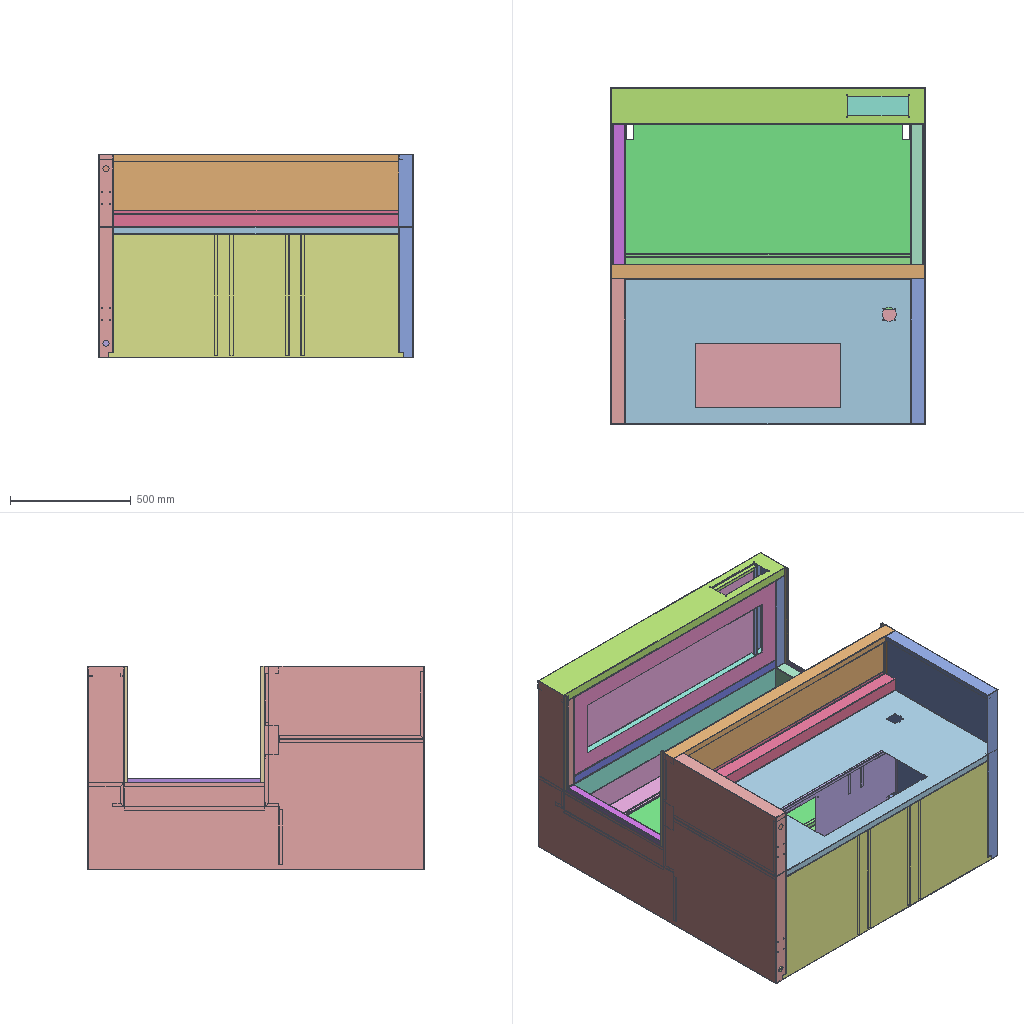Assembly | SolidWorks | 23 different items | 29 placed | box 1300 x 1390 x 840 mm
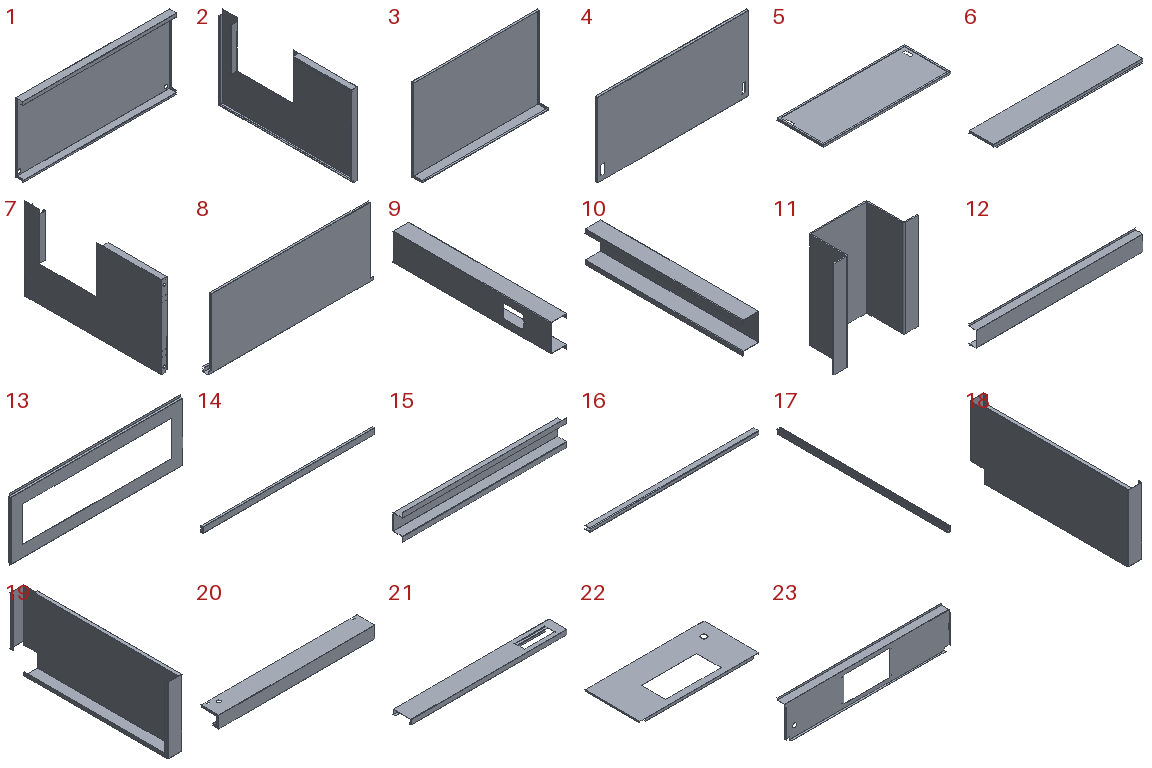Parts list (item | quantity | size | volume | features):
1 | x1 | 1298 x 60 x 593.8 mm | 1188621 mm3 | features EdgeFlange 3, FlatPattern 1, ICE 1, SMBaseFlange 1, SheetMetal 1
2 | x1 | 60 x 1390 x 840 mm | 1426694 mm3 | features EdgeFlange 6, ICE 2, FlatPattern 1, SMBaseFlange 1, SheetMetal 1
3 | x1 | 1220 x 113.8 x 800 mm | 1428081 mm3 | features EdgeFlange 4, FlatPattern 1, ICE 1, SMBaseFlange 1, SheetMetal 1
4 | x1 | 1218 x 20 x 598 mm | 1005424 mm3 | features EdgeFlange 2, FlatPattern 1, SMBaseFlange 1, SheetMetal 1
5 | x1 | 1218 x 448 x 20 mm | 774773 mm3 | features EdgeFlange 2, FlatPattern 1, SMBaseFlange 1, SheetMetal 1
6 | x1 | 1220 x 227.6 x 21.2 mm | 394431 mm3 | features EdgeFlange 3, FlatPattern 1, ICE 1, SMBaseFlange 1, SheetMetal 1
7 | x1 | 60 x 1390 x 840 mm | 1424848 mm3 | features EdgeFlange 6, ICE 3, FlatPattern 1, SMBaseFlange 1, SheetMetal 1
8 | x1 | 1220 x 53.8 x 510 mm | 861259 mm3 | features EdgeFlange 4, ICE 2, FlatPattern 1, SMBaseFlange 1, SheetMetal 1
9 | x1 | 58.8 x 580 x 113.8 mm | 163204 mm3 | features EdgeFlange 2, FlatPattern 1, ICE 1, SMBaseFlange 1, SheetMetal 1
10 | x1 | 58.8 x 580 x 113.8 mm | 163204 mm3 | features EdgeFlange 2, FlatPattern 1, ICE 1, SMBaseFlange 1, SheetMetal 1
11 | x2 | 87.6 x 40 x 100 mm | 19608 mm3 | features EdgeFlange 2, FlatPattern 1, SMBaseFlange 1, SheetMetal 1
12 | x1 | 1298 x 58.8 x 147.6 mm | 406084 mm3 | features EdgeFlange 2, FlatPattern 1, ICE 1, SMBaseFlange 1, SheetMetal 1
13 | x1 | 1180 x 16.2 x 427.6 mm | 373152 mm3 | features EdgeFlange 3, FlatPattern 1, SMBaseFlange 1, SheetMetal 1
14 | x1 | 1180 x 15 x 40 mm | 107252 mm3 | features EdgeFlange 2, FlatPattern 1, SMBaseFlange 1, SheetMetal 1
15 | x2 | 500 x 30 x 77.6 mm | 80038 mm3 | features EdgeFlange 2, FlatPattern 1, SMBaseFlange 1, SheetMetal 1
16 | x4 | 480 x 15 x 10.4 mm | 21369 mm3 | features EdgeFlange 1, FlatPattern 1, SMBaseFlange 1, SheetMetal 1
17 | x2 | 10.4 x 550 x 15 mm | 24485 mm3 | features EdgeFlange 1, FlatPattern 1, SMBaseFlange 1, SheetMetal 1
18 | x1 | 57.6 x 657.6 x 278.8 mm | 314044 mm3 | features EdgeFlange 3, FlatPattern 1, ICE 1, SMBaseFlange 1, SheetMetal 1
19 | x1 | 57.6 x 657.6 x 278.8 mm | 314043 mm3 | features EdgeFlange 3, FlatPattern 1, ICE 1, SMBaseFlange 1, SheetMetal 1
20 | x1 | 1298 x 148.8 x 100 mm | 507645 mm3 | features EdgeFlange 3, ICE 2, FlatPattern 1, SMBaseFlange 1, SheetMetal 1
21 | x1 | 1298 x 150 x 53.8 mm | 411683 mm3 | features EdgeFlange 6, FlatPattern 1, ICE 1, SMBaseFlange 1, SheetMetal 1
22 | x1 | 1298 x 600 x 30 mm | 836579 mm3 | features EdgeFlange 3, ICE 2, FlatPattern 1, SMBaseFlange 1, SheetMetal 1
23 | x1 | 1298 x 73.8 x 275.3 mm | 455986 mm3 | features EdgeFlange 2, ICE 2, FlatPattern 1, SMBaseFlange 1, SheetMetal 1
Mates (type | each side: item.copy, entity, surface, feature):
DistanceDim | 7.1 face plane Base-Flange1 | 2.1 face plane Base-Flange1
Coincident | 7.1 face plane Edge-Flange1 | 2.1 face plane Edge-Flange6 | 2 times
Coincident | 7.1 face plane Base-Flange1 | 21.1 face plane Base-Flange1
Coincident | 7.1 face plane Edge-Flange2 | 21.1 face plane Edge-Flange1
Coincident | 2.1 face plane Base-Flange1 | 21.1 face plane Edge-Flange2
Coincident | 7.1 face plane Edge-Flange2 | 3.1 face plane Base-Flange1
Coincident | 7.1 face plane Edge-Flange3 | 3.1 face plane Edge-Flange2
Coincident | 21.1 face plane Edge-Flange3 | 3.1 face plane Edge-Flange2
Coincident | 2.1 face plane Base-Flange1 | 20.1 face plane Edge-Flange4
Coincident | 3.1 face plane Base-Flange1 | 20.1 face plane Edge-Flange4
DistanceDim | 21.1 face plane Base-Flange1 | 20.1 face plane Base-Flange1
Coincident | 7.1 face plane Edge-Flange1 | 1.1 face plane Edge-Flange1
Coincident | 7.1 face plane Base-Flange1 | 1.1 face plane Edge-Flange3
Coincident | 7.1 face plane Base-Flange1 | 1.1 face plane Base-Flange1
Coincident | 7.1 face plane Base-Flange1 | 23.1 face plane Edge-Flange7
Coincident | 1.1 face plane Base-Flange1 | 23.1 face plane Edge-Flange7
DistanceDim | 2.1 face plane Edge-Flange11 | 23.1 face plane Edge-Flange7
Coincident | 6.1 face plane Base-Flange1 | 3.1 face plane Edge-Flange1
Coincident | 2.1 face plane Edge-Flange13 | 6.1 face plane Edge-Flange2
DistanceDim | 3.1 face plane Edge-Flange3 | 6.1 face plane Edge-Flange1
Coincident | 1.1 face plane Base-Flange1 | 12.1 face plane Edge-Flange2
Coincident | 2.1 face plane Base-Flange1 | 12.1 face plane Base-Flange1
DistanceDim | 12.1 face plane Edge-Flange1 | 1.1 face plane Edge-Flange1
Coincident | 2.1 face plane Base-Flange1 | 22.1 face plane Edge-Flange1
Coincident | 12.1 face plane Base-Flange1 | 22.1 face plane Edge-Flange1
DistanceDim | 22.1 face plane Base-Flange1 | 7.1 face plane Edge-Flange1
Coincident | 7.1 face plane Edge-Flange3 | 8.1 face plane Edge-Flange5
Coincident | 7.1 face plane Edge-Flange1 | 8.1 face plane Edge-Flange5
Coincident | 7.1 face plane Edge-Flange2 | 8.1 face plane Base-Flange2
Coincident | 7.1 face plane Base-Flange1 | 10.1 face plane Edge-Flange2
Coincident | 1.1 face plane Base-Flange1 | 10.1 face plane Edge-Flange2
Coincident | 7.1 face plane Base-Flange1 | 10.1 face plane Edge-Flange1
Coincident | 2.1 face plane Base-Flange1 | 9.1 face plane Edge-Flange2
Coincident | 1.1 face plane Base-Flange1 | 9.1 face plane Edge-Flange2
Coincident | 9.1 face plane Edge-Flange1 | 2.1 face plane Base-Flange1
Coincident | 1.1 face plane Base-Flange1 | 19.1 face plane Edge-Flange2
Coincident | 22.1 face plane Base-Flange1 | 19.1 face plane Edge-Flange2
Coincident | 7.1 face plane Edge-Flange3 | 19.1 face plane Base-Flange1
Coincident | 20.1 face plane Base-Flange1 | 14.1 face plane Edge-Flange1
Coincident | 20.1 face plane Edge-Flange2 | 14.1 face plane Base-Flange1
Coincident | 2.1 face plane Edge-Flange16 | 14.1 face plane Edge-Flange1
Coincident | 8.1 face plane Edge-Flange5 | 15.1 face plane Edge-Flange2
Coincident | 8.1 face plane Edge-Flange8 | 15.1 face plane Edge-Flange1
Coincident | 15.1 face plane Base-Flange1 | 15.2 face plane Base-Flange1
Coincident | 8.1 face plane Edge-Flange8 | 15.2 edge
Coincident | 2.1 face plane Edge-Flange16 | 13.1 face plane Edge-Flange1
Coincident | 21.1 face plane Edge-Flange2 | 13.1 face plane Base-Flange1
Coincident | 1.1 face plane Edge-Flange3 | 11.1 face plane Base-Flange1
Coincident | 23.1 face plane Base-Flange1 | 11.1 face plane Edge-Flange2
DistanceDim | 11.1 face plane Edge-Flange1 | 7.1 face plane Base-Flange1
Coincident | 11.1 face plane Base-Flange1 | 11.2 face plane Base-Flange1
Coincident | 11.1 face plane Edge-Flange1 | 11.2 face plane Edge-Flange1
DistanceDim | 2.1 face plane Base-Flange1 | 11.2 face plane Edge-Flange1
Coincident | 16.1 face plane Edge-Flange1 | 2.1 face plane Base-Flange1
Coincident | 1.1 face plane Base-Flange1 | 16.1 face plane Base-Flange1
Coincident | 1.1 face plane Edge-Flange1 | 16.1 face plane Base-Flange1
Coincident | 16.2 face plane Base-Flange1 | 2.1 face plane Edge-Flange6
Coincident | 2.1 face plane Base-Flange1 | 16.2 face plane Edge-Flange1
Coincident | 21.1 face plane Base-Flange1 | 16.2 face plane Edge-Flange1
Coincident | 7.1 face plane Edge-Flange1 | 16.3 face plane Base-Flange1
Coincident | 7.1 face plane Base-Flange1 | 16.3 face plane Edge-Flange1
Coincident | 21.1 face plane Base-Flange1 | 16.3 face plane Edge-Flange1
Coincident | 1.1 face plane Base-Flange1 | 16.4 face plane Base-Flange1
Coincident | 7.1 face plane Base-Flange1 | 16.4 face plane Edge-Flange1
Coincident | 10.1 face plane Edge-Flange1 | 16.4 face plane Edge-Flange1
Coincident | 2.1 face plane Base-Flange1 | 17.1 face plane Edge-Flange1
Coincident | 16.2 face plane Edge-Flange1 | 17.1 face plane Base-Flange1
Coincident | 9.1 face plane Edge-Flange1 | 17.1 face plane Base-Flange1
Coincident | 16.3 face plane Edge-Flange1 | 17.2 face plane Edge-Flange1
Coincident | 7.1 face plane Base-Flange1 | 17.2 face plane Edge-Flange1
Coincident | 10.1 face plane Edge-Flange1 | 17.2 face plane Base-Flange1
Coincident | 3.1 face plane Edge-Flange1 | 4.1 face plane Base-Flange1
DistanceDim | 4.1 face plane Edge-Flange1 | 2.1 face plane Edge-Flange13
DistanceDim | 4.1 face plane Edge-Flange1 | 6.1 face plane Edge-Flange1
Coincident | 6.1 face plane Edge-Flange3 | 5.1 face plane Edge-Flange2
DistanceDim | 7.1 face plane Edge-Flange3 | 5.1 face plane Edge-Flange1
DistanceDim | 5.1 face plane Edge-Flange1 | 8.1 face plane Edge-Flange6
Coincident | 21.1 face plane Edge-Flange5 | 13.1 face plane Edge-Flange1